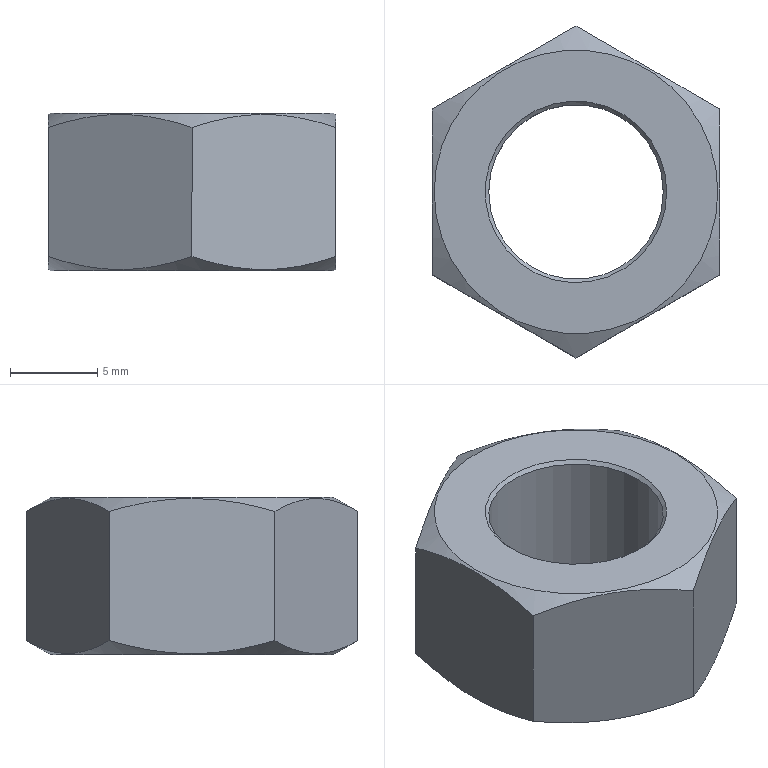Part | STEP file | N1101210 | 1 solid | 13 faces | box 16.454 x 19 x 9 mm | volume 1389 mm3 | plane 8 | cone 4 | cylinder 1 | commonest cylinder face diameters 10 x1